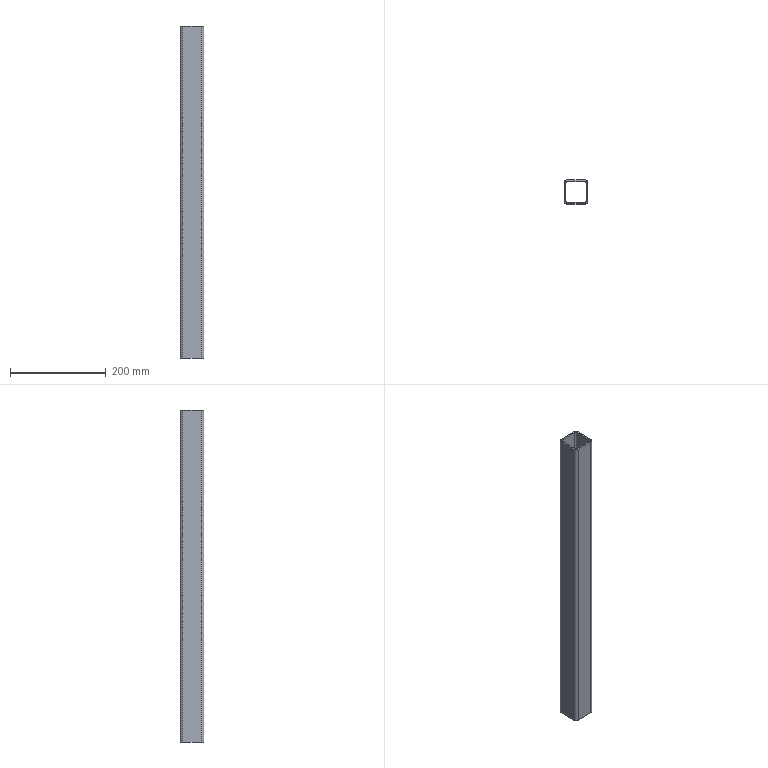Part | SolidWorks | 1 solid | 18 faces | box 50 x 50 x 695 mm | volume 375872 mm3 | plane 10 | cylinder 8 | commonest cylinder face diameters 6 x4 12 x4
STEP:
#1=CARTESIAN_POINT('',(19.,25.,347.5));
#2=VERTEX_POINT('',#1);
#3=CARTESIAN_POINT('',(25.,19.,347.5));
#4=VERTEX_POINT('',#3);
#5=CARTESIAN_POINT('',(19.,19.,347.5));
#6=DIRECTION('',(0.,0.,-1.));
#7=DIRECTION('',(-1.,0.,0.));
#8=AXIS2_PLACEMENT_3D('',#5,#6,#7);
#9=CIRCLE('',#8,6.);
#10=EDGE_CURVE('',#2,#4,#9,.T.);
#11=ORIENTED_EDGE('',*,*,#10,.T.);
#12=CARTESIAN_POINT('',(25.,19.,-347.5));
#13=VERTEX_POINT('',#12);
#14=CARTESIAN_POINT('',(25.,19.,-347.5));
#15=DIRECTION('',(0.,0.,1.));
#16=VECTOR('',#15,1000.);
#17=LINE('',#14,#16);
#18=EDGE_CURVE('',#13,#4,#17,.T.);
#19=ORIENTED_EDGE('',*,*,#18,.F.);
#20=CARTESIAN_POINT('',(19.,25.,-347.5));
#21=VERTEX_POINT('',#20);
#22=CARTESIAN_POINT('',(19.,19.,-347.5));
#23=DIRECTION('',(0.,0.,-1.));
#24=DIRECTION('',(-1.,0.,0.));
#25=AXIS2_PLACEMENT_3D('',#22,#23,#24);
#26=CIRCLE('',#25,6.);
#27=EDGE_CURVE('',#21,#13,#26,.T.);
#28=ORIENTED_EDGE('',*,*,#27,.F.);
#29=CARTESIAN_POINT('',(19.,25.,-347.5));
#30=DIRECTION('',(0.,0.,1.));
#31=VECTOR('',#30,1000.);
#32=LINE('',#29,#31);
#33=EDGE_CURVE('',#21,#2,#32,.T.);
#34=ORIENTED_EDGE('',*,*,#33,.T.);
#35=EDGE_LOOP('',(#11,#19,#28,#34));
#36=FACE_OUTER_BOUND('',#35,.T.);
#37=CARTESIAN_POINT('',(19.,19.,-347.5));
#38=DIRECTION('',(0.,0.,1.));
#39=DIRECTION('',(1.,0.,0.));
#40=AXIS2_PLACEMENT_3D('',#37,#38,#39);
#41=CYLINDRICAL_SURFACE('',#40,6.);
#42=ADVANCED_FACE('',(#36),#41,.T.);
#43=CARTESIAN_POINT('',(25.,-19.,347.5));
#44=VERTEX_POINT('',#43);
#45=CARTESIAN_POINT('',(25.,19.,347.5));
#46=DIRECTION('',(0.,-1.,0.));
#47=VECTOR('',#46,1000.);
#48=LINE('',#45,#47);
#49=EDGE_CURVE('',#4,#44,#48,.T.);
#50=ORIENTED_EDGE('',*,*,#49,.T.);
#51=CARTESIAN_POINT('',(25.,-19.,-347.5));
#52=VERTEX_POINT('',#51);
#53=CARTESIAN_POINT('',(25.,-19.,-347.5));
#54=DIRECTION('',(0.,0.,1.));
#55=VECTOR('',#54,1000.);
#56=LINE('',#53,#55);
#57=EDGE_CURVE('',#52,#44,#56,.T.);
#58=ORIENTED_EDGE('',*,*,#57,.F.);
#59=CARTESIAN_POINT('',(25.,19.,-347.5));
#60=DIRECTION('',(0.,-1.,0.));
#61=VECTOR('',#60,1000.);
#62=LINE('',#59,#61);
#63=EDGE_CURVE('',#13,#52,#62,.T.);
#64=ORIENTED_EDGE('',*,*,#63,.F.);
#65=ORIENTED_EDGE('',*,*,#18,.T.);
#66=EDGE_LOOP('',(#50,#58,#64,#65));
#67=FACE_OUTER_BOUND('',#66,.T.);
#68=CARTESIAN_POINT('',(25.,19.,-347.5));
#69=DIRECTION('',(-1.,0.,0.));
#70=DIRECTION('',(0.,0.,1.));
#71=AXIS2_PLACEMENT_3D('',#68,#69,#70);
#72=PLANE('',#71);
#73=ADVANCED_FACE('',(#67),#72,.F.);
#74=CARTESIAN_POINT('',(19.,-25.,347.5));
#75=VERTEX_POINT('',#74);
#76=CARTESIAN_POINT('',(19.,-19.,347.5));
#77=DIRECTION('',(0.,0.,-1.));
#78=DIRECTION('',(-1.,0.,0.));
#79=AXIS2_PLACEMENT_3D('',#76,#77,#78);
#80=CIRCLE('',#79,6.);
#81=EDGE_CURVE('',#44,#75,#80,.T.);
#82=ORIENTED_EDGE('',*,*,#81,.T.);
#83=CARTESIAN_POINT('',(19.,-25.,-347.5));
#84=VERTEX_POINT('',#83);
#85=CARTESIAN_POINT('',(19.,-25.,-347.5));
#86=DIRECTION('',(0.,0.,1.));
#87=VECTOR('',#86,1000.);
#88=LINE('',#85,#87);
#89=EDGE_CURVE('',#84,#75,#88,.T.);
#90=ORIENTED_EDGE('',*,*,#89,.F.);
#91=CARTESIAN_POINT('',(19.,-19.,-347.5));
#92=DIRECTION('',(0.,0.,-1.));
#93=DIRECTION('',(-1.,0.,0.));
#94=AXIS2_PLACEMENT_3D('',#91,#92,#93);
#95=CIRCLE('',#94,6.);
#96=EDGE_CURVE('',#52,#84,#95,.T.);
#97=ORIENTED_EDGE('',*,*,#96,.F.);
#98=ORIENTED_EDGE('',*,*,#57,.T.);
#99=EDGE_LOOP('',(#82,#90,#97,#98));
#100=FACE_OUTER_BOUND('',#99,.T.);
#101=CARTESIAN_POINT('',(19.,-19.,-347.5));
#102=DIRECTION('',(0.,0.,1.));
#103=DIRECTION('',(1.,0.,0.));
#104=AXIS2_PLACEMENT_3D('',#101,#102,#103);
#105=CYLINDRICAL_SURFACE('',#104,6.);
#106=ADVANCED_FACE('',(#100),#105,.T.);
#107=CARTESIAN_POINT('',(-19.,-25.,347.5));
#108=VERTEX_POINT('',#107);
#109=CARTESIAN_POINT('',(-19.,-25.,347.5));
#110=DIRECTION('',(-1.,0.,0.));
#111=VECTOR('',#110,1000.);
#112=LINE('',#109,#111);
#113=EDGE_CURVE('',#75,#108,#112,.T.);
#114=ORIENTED_EDGE('',*,*,#113,.T.);
#115=CARTESIAN_POINT('',(-19.,-25.,-347.5));
#116=VERTEX_POINT('',#115);
#117=CARTESIAN_POINT('',(-19.,-25.,-347.5));
#118=DIRECTION('',(0.,0.,1.));
#119=VECTOR('',#118,1000.);
#120=LINE('',#117,#119);
#121=EDGE_CURVE('',#116,#108,#120,.T.);
#122=ORIENTED_EDGE('',*,*,#121,.F.);
#123=CARTESIAN_POINT('',(-19.,-25.,-347.5));
#124=DIRECTION('',(-1.,0.,0.));
#125=VECTOR('',#124,1000.);
#126=LINE('',#123,#125);
#127=EDGE_CURVE('',#84,#116,#126,.T.);
#128=ORIENTED_EDGE('',*,*,#127,.F.);
#129=ORIENTED_EDGE('',*,*,#89,.T.);
#130=EDGE_LOOP('',(#114,#122,#128,#129));
#131=FACE_OUTER_BOUND('',#130,.T.);
#132=CARTESIAN_POINT('',(-19.,-25.,-347.5));
#133=DIRECTION('',(0.,1.,0.));
#134=DIRECTION('',(0.,0.,1.));
#135=AXIS2_PLACEMENT_3D('',#132,#133,#134);
#136=PLANE('',#135);
#137=ADVANCED_FACE('',(#131),#136,.F.);
#138=CARTESIAN_POINT('',(-25.,-19.,347.5));
#139=VERTEX_POINT('',#138);
#140=CARTESIAN_POINT('',(-19.,-19.,347.5));
#141=DIRECTION('',(0.,0.,-1.));
#142=DIRECTION('',(-1.,0.,0.));
#143=AXIS2_PLACEMENT_3D('',#140,#141,#142);
#144=CIRCLE('',#143,6.);
#145=EDGE_CURVE('',#108,#139,#144,.T.);
#146=ORIENTED_EDGE('',*,*,#145,.T.);
#147=CARTESIAN_POINT('',(-25.,-19.,-347.5));
#148=VERTEX_POINT('',#147);
#149=CARTESIAN_POINT('',(-25.,-19.,-347.5));
#150=DIRECTION('',(0.,0.,1.));
#151=VECTOR('',#150,1000.);
#152=LINE('',#149,#151);
#153=EDGE_CURVE('',#148,#139,#152,.T.);
#154=ORIENTED_EDGE('',*,*,#153,.F.);
#155=CARTESIAN_POINT('',(-19.,-19.,-347.5));
#156=DIRECTION('',(0.,0.,-1.));
#157=DIRECTION('',(-1.,0.,0.));
#158=AXIS2_PLACEMENT_3D('',#155,#156,#157);
#159=CIRCLE('',#158,6.);
#160=EDGE_CURVE('',#116,#148,#159,.T.);
#161=ORIENTED_EDGE('',*,*,#160,.F.);
#162=ORIENTED_EDGE('',*,*,#121,.T.);
#163=EDGE_LOOP('',(#146,#154,#161,#162));
#164=FACE_OUTER_BOUND('',#163,.T.);
#165=CARTESIAN_POINT('',(-19.,-19.,-347.5));
#166=DIRECTION('',(0.,0.,1.));
#167=DIRECTION('',(1.,0.,0.));
#168=AXIS2_PLACEMENT_3D('',#165,#166,#167);
#169=CYLINDRICAL_SURFACE('',#168,6.);
#170=ADVANCED_FACE('',(#164),#169,.T.);
#171=CARTESIAN_POINT('',(-25.,19.,347.5));
#172=VERTEX_POINT('',#171);
#173=CARTESIAN_POINT('',(-25.,-19.,347.5));
#174=DIRECTION('',(0.,1.,0.));
#175=VECTOR('',#174,1000.);
#176=LINE('',#173,#175);
#177=EDGE_CURVE('',#139,#172,#176,.T.);
#178=ORIENTED_EDGE('',*,*,#177,.T.);
#179=CARTESIAN_POINT('',(-25.,19.,-347.5));
#180=VERTEX_POINT('',#179);
#181=CARTESIAN_POINT('',(-25.,19.,-347.5));
#182=DIRECTION('',(0.,0.,1.));
#183=VECTOR('',#182,1000.);
#184=LINE('',#181,#183);
#185=EDGE_CURVE('',#180,#172,#184,.T.);
#186=ORIENTED_EDGE('',*,*,#185,.F.);
#187=CARTESIAN_POINT('',(-25.,-19.,-347.5));
#188=DIRECTION('',(0.,1.,0.));
#189=VECTOR('',#188,1000.);
#190=LINE('',#187,#189);
#191=EDGE_CURVE('',#148,#180,#190,.T.);
#192=ORIENTED_EDGE('',*,*,#191,.F.);
#193=ORIENTED_EDGE('',*,*,#153,.T.);
#194=EDGE_LOOP('',(#178,#186,#192,#193));
#195=FACE_OUTER_BOUND('',#194,.T.);
#196=CARTESIAN_POINT('',(-25.,-19.,-347.5));
#197=DIRECTION('',(1.,0.,0.));
#198=DIRECTION('',(0.,0.,-1.));
#199=AXIS2_PLACEMENT_3D('',#196,#197,#198);
#200=PLANE('',#199);
#201=ADVANCED_FACE('',(#195),#200,.F.);
#202=CARTESIAN_POINT('',(-19.,25.,347.5));
#203=VERTEX_POINT('',#202);
#204=CARTESIAN_POINT('',(-19.,19.,347.5));
#205=DIRECTION('',(0.,0.,-1.));
#206=DIRECTION('',(-1.,0.,0.));
#207=AXIS2_PLACEMENT_3D('',#204,#205,#206);
#208=CIRCLE('',#207,6.);
#209=EDGE_CURVE('',#172,#203,#208,.T.);
#210=ORIENTED_EDGE('',*,*,#209,.T.);
#211=CARTESIAN_POINT('',(-19.,25.,-347.5));
#212=VERTEX_POINT('',#211);
#213=CARTESIAN_POINT('',(-19.,25.,-347.5));
#214=DIRECTION('',(0.,0.,1.));
#215=VECTOR('',#214,1000.);
#216=LINE('',#213,#215);
#217=EDGE_CURVE('',#212,#203,#216,.T.);
#218=ORIENTED_EDGE('',*,*,#217,.F.);
#219=CARTESIAN_POINT('',(-19.,19.,-347.5));
#220=DIRECTION('',(0.,0.,-1.));
#221=DIRECTION('',(-1.,0.,0.));
#222=AXIS2_PLACEMENT_3D('',#219,#220,#221);
#223=CIRCLE('',#222,6.);
#224=EDGE_CURVE('',#180,#212,#223,.T.);
#225=ORIENTED_EDGE('',*,*,#224,.F.);
#226=ORIENTED_EDGE('',*,*,#185,.T.);
#227=EDGE_LOOP('',(#210,#218,#225,#226));
#228=FACE_OUTER_BOUND('',#227,.T.);
#229=CARTESIAN_POINT('',(-19.,19.,-347.5));
#230=DIRECTION('',(0.,0.,1.));
#231=DIRECTION('',(1.,0.,0.));
#232=AXIS2_PLACEMENT_3D('',#229,#230,#231);
#233=CYLINDRICAL_SURFACE('',#232,6.);
#234=ADVANCED_FACE('',(#228),#233,.T.);
#235=CARTESIAN_POINT('',(22.,-19.,347.5));
#236=VERTEX_POINT('',#235);
#237=CARTESIAN_POINT('',(19.,-22.,347.5));
#238=VERTEX_POINT('',#237);
#239=CARTESIAN_POINT('',(19.,-19.,347.5));
#240=DIRECTION('',(0.,0.,-1.));
#241=DIRECTION('',(-1.,0.,0.));
#242=AXIS2_PLACEMENT_3D('',#239,#240,#241);
#243=CIRCLE('',#242,3.);
#244=EDGE_CURVE('',#236,#238,#243,.T.);
#245=ORIENTED_EDGE('',*,*,#244,.F.);
#246=CARTESIAN_POINT('',(22.,-19.,-347.5));
#247=VERTEX_POINT('',#246);
#248=CARTESIAN_POINT('',(22.,-19.,-347.5));
#249=DIRECTION('',(0.,0.,1.));
#250=VECTOR('',#249,1000.);
#251=LINE('',#248,#250);
#252=EDGE_CURVE('',#247,#236,#251,.T.);
#253=ORIENTED_EDGE('',*,*,#252,.F.);
#254=CARTESIAN_POINT('',(19.,-22.,-347.5));
#255=VERTEX_POINT('',#254);
#256=CARTESIAN_POINT('',(19.,-19.,-347.5));
#257=DIRECTION('',(0.,0.,-1.));
#258=DIRECTION('',(-1.,0.,0.));
#259=AXIS2_PLACEMENT_3D('',#256,#257,#258);
#260=CIRCLE('',#259,3.);
#261=EDGE_CURVE('',#247,#255,#260,.T.);
#262=ORIENTED_EDGE('',*,*,#261,.T.);
#263=CARTESIAN_POINT('',(19.,-22.,-347.5));
#264=DIRECTION('',(0.,0.,1.));
#265=VECTOR('',#264,1000.);
#266=LINE('',#263,#265);
#267=EDGE_CURVE('',#255,#238,#266,.T.);
#268=ORIENTED_EDGE('',*,*,#267,.T.);
#269=EDGE_LOOP('',(#245,#253,#262,#268));
#270=FACE_OUTER_BOUND('',#269,.T.);
#271=CARTESIAN_POINT('',(19.,-19.,-347.5));
#272=DIRECTION('',(0.,0.,1.));
#273=DIRECTION('',(1.,0.,0.));
#274=AXIS2_PLACEMENT_3D('',#271,#272,#273);
#275=CYLINDRICAL_SURFACE('',#274,3.);
#276=ADVANCED_FACE('',(#270),#275,.F.);
#277=CARTESIAN_POINT('',(22.,19.,347.5));
#278=VERTEX_POINT('',#277);
#279=CARTESIAN_POINT('',(22.,19.,347.5));
#280=DIRECTION('',(0.,-1.,0.));
#281=VECTOR('',#280,1000.);
#282=LINE('',#279,#281);
#283=EDGE_CURVE('',#278,#236,#282,.T.);
#284=ORIENTED_EDGE('',*,*,#283,.F.);
#285=CARTESIAN_POINT('',(22.,19.,-347.5));
#286=VERTEX_POINT('',#285);
#287=CARTESIAN_POINT('',(22.,19.,-347.5));
#288=DIRECTION('',(0.,0.,1.));
#289=VECTOR('',#288,1000.);
#290=LINE('',#287,#289);
#291=EDGE_CURVE('',#286,#278,#290,.T.);
#292=ORIENTED_EDGE('',*,*,#291,.F.);
#293=CARTESIAN_POINT('',(22.,19.,-347.5));
#294=DIRECTION('',(0.,-1.,0.));
#295=VECTOR('',#294,1000.);
#296=LINE('',#293,#295);
#297=EDGE_CURVE('',#286,#247,#296,.T.);
#298=ORIENTED_EDGE('',*,*,#297,.T.);
#299=ORIENTED_EDGE('',*,*,#252,.T.);
#300=EDGE_LOOP('',(#284,#292,#298,#299));
#301=FACE_OUTER_BOUND('',#300,.T.);
#302=CARTESIAN_POINT('',(22.,19.,-347.5));
#303=DIRECTION('',(-1.,0.,0.));
#304=DIRECTION('',(0.,0.,1.));
#305=AXIS2_PLACEMENT_3D('',#302,#303,#304);
#306=PLANE('',#305);
#307=ADVANCED_FACE('',(#301),#306,.T.);
#308=CARTESIAN_POINT('',(19.,22.,347.5));
#309=VERTEX_POINT('',#308);
#310=CARTESIAN_POINT('',(19.,19.,347.5));
#311=DIRECTION('',(0.,0.,-1.));
#312=DIRECTION('',(-1.,0.,0.));
#313=AXIS2_PLACEMENT_3D('',#310,#311,#312);
#314=CIRCLE('',#313,3.);
#315=EDGE_CURVE('',#309,#278,#314,.T.);
#316=ORIENTED_EDGE('',*,*,#315,.F.);
#317=CARTESIAN_POINT('',(19.,22.,-347.5));
#318=VERTEX_POINT('',#317);
#319=CARTESIAN_POINT('',(19.,22.,-347.5));
#320=DIRECTION('',(0.,0.,1.));
#321=VECTOR('',#320,1000.);
#322=LINE('',#319,#321);
#323=EDGE_CURVE('',#318,#309,#322,.T.);
#324=ORIENTED_EDGE('',*,*,#323,.F.);
#325=CARTESIAN_POINT('',(19.,19.,-347.5));
#326=DIRECTION('',(0.,0.,-1.));
#327=DIRECTION('',(-1.,0.,0.));
#328=AXIS2_PLACEMENT_3D('',#325,#326,#327);
#329=CIRCLE('',#328,3.);
#330=EDGE_CURVE('',#318,#286,#329,.T.);
#331=ORIENTED_EDGE('',*,*,#330,.T.);
#332=ORIENTED_EDGE('',*,*,#291,.T.);
#333=EDGE_LOOP('',(#316,#324,#331,#332));
#334=FACE_OUTER_BOUND('',#333,.T.);
#335=CARTESIAN_POINT('',(19.,19.,-347.5));
#336=DIRECTION('',(0.,0.,1.));
#337=DIRECTION('',(1.,0.,0.));
#338=AXIS2_PLACEMENT_3D('',#335,#336,#337);
#339=CYLINDRICAL_SURFACE('',#338,3.);
#340=ADVANCED_FACE('',(#334),#339,.F.);
#341=CARTESIAN_POINT('',(-19.,22.,347.5));
#342=VERTEX_POINT('',#341);
#343=CARTESIAN_POINT('',(19.,22.,347.5));
#344=DIRECTION('',(1.,0.,0.));
#345=VECTOR('',#344,1000.);
#346=LINE('',#343,#345);
#347=EDGE_CURVE('',#342,#309,#346,.T.);
#348=ORIENTED_EDGE('',*,*,#347,.F.);
#349=CARTESIAN_POINT('',(-19.,22.,-347.5));
#350=VERTEX_POINT('',#349);
#351=CARTESIAN_POINT('',(-19.,22.,-347.5));
#352=DIRECTION('',(0.,0.,1.));
#353=VECTOR('',#352,1000.);
#354=LINE('',#351,#353);
#355=EDGE_CURVE('',#350,#342,#354,.T.);
#356=ORIENTED_EDGE('',*,*,#355,.F.);
#357=CARTESIAN_POINT('',(19.,22.,-347.5));
#358=DIRECTION('',(1.,0.,0.));
#359=VECTOR('',#358,1000.);
#360=LINE('',#357,#359);
#361=EDGE_CURVE('',#350,#318,#360,.T.);
#362=ORIENTED_EDGE('',*,*,#361,.T.);
#363=ORIENTED_EDGE('',*,*,#323,.T.);
#364=EDGE_LOOP('',(#348,#356,#362,#363));
#365=FACE_OUTER_BOUND('',#364,.T.);
#366=CARTESIAN_POINT('',(19.,22.,-347.5));
#367=DIRECTION('',(0.,-1.,0.));
#368=DIRECTION('',(0.,0.,-1.));
#369=AXIS2_PLACEMENT_3D('',#366,#367,#368);
#370=PLANE('',#369);
#371=ADVANCED_FACE('',(#365),#370,.T.);
#372=CARTESIAN_POINT('',(-22.,19.,347.5));
#373=VERTEX_POINT('',#372);
#374=CARTESIAN_POINT('',(-19.,19.,347.5));
#375=DIRECTION('',(0.,0.,-1.));
#376=DIRECTION('',(-1.,0.,0.));
#377=AXIS2_PLACEMENT_3D('',#374,#375,#376);
#378=CIRCLE('',#377,3.);
#379=EDGE_CURVE('',#373,#342,#378,.T.);
#380=ORIENTED_EDGE('',*,*,#379,.F.);
#381=CARTESIAN_POINT('',(-22.,19.,-347.5));
#382=VERTEX_POINT('',#381);
#383=CARTESIAN_POINT('',(-22.,19.,-347.5));
#384=DIRECTION('',(0.,0.,1.));
#385=VECTOR('',#384,1000.);
#386=LINE('',#383,#385);
#387=EDGE_CURVE('',#382,#373,#386,.T.);
#388=ORIENTED_EDGE('',*,*,#387,.F.);
#389=CARTESIAN_POINT('',(-19.,19.,-347.5));
#390=DIRECTION('',(0.,0.,-1.));
#391=DIRECTION('',(-1.,0.,0.));
#392=AXIS2_PLACEMENT_3D('',#389,#390,#391);
#393=CIRCLE('',#392,3.);
#394=EDGE_CURVE('',#382,#350,#393,.T.);
#395=ORIENTED_EDGE('',*,*,#394,.T.);
#396=ORIENTED_EDGE('',*,*,#355,.T.);
#397=EDGE_LOOP('',(#380,#388,#395,#396));
#398=FACE_OUTER_BOUND('',#397,.T.);
#399=CARTESIAN_POINT('',(-19.,19.,-347.5));
#400=DIRECTION('',(0.,0.,1.));
#401=DIRECTION('',(1.,0.,0.));
#402=AXIS2_PLACEMENT_3D('',#399,#400,#401);
#403=CYLINDRICAL_SURFACE('',#402,3.);
#404=ADVANCED_FACE('',(#398),#403,.F.);
#405=CARTESIAN_POINT('',(-22.,-19.,347.5));
#406=VERTEX_POINT('',#405);
#407=CARTESIAN_POINT('',(-22.,-19.,347.5));
#408=DIRECTION('',(0.,1.,0.));
#409=VECTOR('',#408,1000.);
#410=LINE('',#407,#409);
#411=EDGE_CURVE('',#406,#373,#410,.T.);
#412=ORIENTED_EDGE('',*,*,#411,.F.);
#413=CARTESIAN_POINT('',(-22.,-19.,-347.5));
#414=VERTEX_POINT('',#413);
#415=CARTESIAN_POINT('',(-22.,-19.,-347.5));
#416=DIRECTION('',(0.,0.,1.));
#417=VECTOR('',#416,1000.);
#418=LINE('',#415,#417);
#419=EDGE_CURVE('',#414,#406,#418,.T.);
#420=ORIENTED_EDGE('',*,*,#419,.F.);
#421=CARTESIAN_POINT('',(-22.,-19.,-347.5));
#422=DIRECTION('',(0.,1.,0.));
#423=VECTOR('',#422,1000.);
#424=LINE('',#421,#423);
#425=EDGE_CURVE('',#414,#382,#424,.T.);
#426=ORIENTED_EDGE('',*,*,#425,.T.);
#427=ORIENTED_EDGE('',*,*,#387,.T.);
#428=EDGE_LOOP('',(#412,#420,#426,#427));
#429=FACE_OUTER_BOUND('',#428,.T.);
#430=CARTESIAN_POINT('',(-22.,-19.,-347.5));
#431=DIRECTION('',(1.,0.,0.));
#432=DIRECTION('',(0.,0.,-1.));
#433=AXIS2_PLACEMENT_3D('',#430,#431,#432);
#434=PLANE('',#433);
#435=ADVANCED_FACE('',(#429),#434,.T.);
#436=CARTESIAN_POINT('',(-19.,-22.,347.5));
#437=VERTEX_POINT('',#436);
#438=CARTESIAN_POINT('',(-19.,-19.,347.5));
#439=DIRECTION('',(0.,0.,-1.));
#440=DIRECTION('',(-1.,0.,0.));
#441=AXIS2_PLACEMENT_3D('',#438,#439,#440);
#442=CIRCLE('',#441,3.);
#443=EDGE_CURVE('',#437,#406,#442,.T.);
#444=ORIENTED_EDGE('',*,*,#443,.F.);
#445=CARTESIAN_POINT('',(-19.,-22.,-347.5));
#446=VERTEX_POINT('',#445);
#447=CARTESIAN_POINT('',(-19.,-22.,-347.5));
#448=DIRECTION('',(0.,0.,1.));
#449=VECTOR('',#448,1000.);
#450=LINE('',#447,#449);
#451=EDGE_CURVE('',#446,#437,#450,.T.);
#452=ORIENTED_EDGE('',*,*,#451,.F.);
#453=CARTESIAN_POINT('',(-19.,-19.,-347.5));
#454=DIRECTION('',(0.,0.,-1.));
#455=DIRECTION('',(-1.,0.,0.));
#456=AXIS2_PLACEMENT_3D('',#453,#454,#455);
#457=CIRCLE('',#456,3.);
#458=EDGE_CURVE('',#446,#414,#457,.T.);
#459=ORIENTED_EDGE('',*,*,#458,.T.);
#460=ORIENTED_EDGE('',*,*,#419,.T.);
#461=EDGE_LOOP('',(#444,#452,#459,#460));
#462=FACE_OUTER_BOUND('',#461,.T.);
#463=CARTESIAN_POINT('',(-19.,-19.,-347.5));
#464=DIRECTION('',(0.,0.,1.));
#465=DIRECTION('',(1.,0.,0.));
#466=AXIS2_PLACEMENT_3D('',#463,#464,#465);
#467=CYLINDRICAL_SURFACE('',#466,3.);
#468=ADVANCED_FACE('',(#462),#467,.F.);
#469=CARTESIAN_POINT('',(-19.,-22.,347.5));
#470=DIRECTION('',(-1.,0.,0.));
#471=VECTOR('',#470,1000.);
#472=LINE('',#469,#471);
#473=EDGE_CURVE('',#238,#437,#472,.T.);
#474=ORIENTED_EDGE('',*,*,#473,.F.);
#475=ORIENTED_EDGE('',*,*,#267,.F.);
#476=CARTESIAN_POINT('',(-19.,-22.,-347.5));
#477=DIRECTION('',(-1.,0.,0.));
#478=VECTOR('',#477,1000.);
#479=LINE('',#476,#478);
#480=EDGE_CURVE('',#255,#446,#479,.T.);
#481=ORIENTED_EDGE('',*,*,#480,.T.);
#482=ORIENTED_EDGE('',*,*,#451,.T.);
#483=EDGE_LOOP('',(#474,#475,#481,#482));
#484=FACE_OUTER_BOUND('',#483,.T.);
#485=CARTESIAN_POINT('',(-19.,-22.,-347.5));
#486=DIRECTION('',(0.,1.,0.));
#487=DIRECTION('',(0.,0.,1.));
#488=AXIS2_PLACEMENT_3D('',#485,#486,#487);
#489=PLANE('',#488);
#490=ADVANCED_FACE('',(#484),#489,.T.);
#491=CARTESIAN_POINT('',(19.,25.,347.5));
#492=DIRECTION('',(1.,0.,0.));
#493=VECTOR('',#492,1000.);
#494=LINE('',#491,#493);
#495=EDGE_CURVE('',#203,#2,#494,.T.);
#496=ORIENTED_EDGE('',*,*,#495,.T.);
#497=ORIENTED_EDGE('',*,*,#33,.F.);
#498=CARTESIAN_POINT('',(19.,25.,-347.5));
#499=DIRECTION('',(1.,0.,0.));
#500=VECTOR('',#499,1000.);
#501=LINE('',#498,#500);
#502=EDGE_CURVE('',#212,#21,#501,.T.);
#503=ORIENTED_EDGE('',*,*,#502,.F.);
#504=ORIENTED_EDGE('',*,*,#217,.T.);
#505=EDGE_LOOP('',(#496,#497,#503,#504));
#506=FACE_OUTER_BOUND('',#505,.T.);
#507=CARTESIAN_POINT('',(19.,25.,-347.5));
#508=DIRECTION('',(0.,-1.,0.));
#509=DIRECTION('',(0.,0.,-1.));
#510=AXIS2_PLACEMENT_3D('',#507,#508,#509);
#511=PLANE('',#510);
#512=ADVANCED_FACE('',(#506),#511,.F.);
#513=ORIENTED_EDGE('',*,*,#261,.F.);
#514=ORIENTED_EDGE('',*,*,#297,.F.);
#515=ORIENTED_EDGE('',*,*,#330,.F.);
#516=ORIENTED_EDGE('',*,*,#361,.F.);
#517=ORIENTED_EDGE('',*,*,#394,.F.);
#518=ORIENTED_EDGE('',*,*,#425,.F.);
#519=ORIENTED_EDGE('',*,*,#458,.F.);
#520=ORIENTED_EDGE('',*,*,#480,.F.);
#521=EDGE_LOOP('',(#513,#514,#515,#516,#517,#518,#519,#520));
#522=FACE_BOUND('',#521,.T.);
#523=ORIENTED_EDGE('',*,*,#27,.T.);
#524=ORIENTED_EDGE('',*,*,#63,.T.);
#525=ORIENTED_EDGE('',*,*,#96,.T.);
#526=ORIENTED_EDGE('',*,*,#127,.T.);
#527=ORIENTED_EDGE('',*,*,#160,.T.);
#528=ORIENTED_EDGE('',*,*,#191,.T.);
#529=ORIENTED_EDGE('',*,*,#224,.T.);
#530=ORIENTED_EDGE('',*,*,#502,.T.);
#531=EDGE_LOOP('',(#523,#524,#525,#526,#527,#528,#529,#530));
#532=FACE_OUTER_BOUND('',#531,.T.);
#533=CARTESIAN_POINT('',(19.,19.,-347.5));
#534=DIRECTION('',(0.,0.,-1.));
#535=DIRECTION('',(-1.,0.,0.));
#536=AXIS2_PLACEMENT_3D('',#533,#534,#535);
#537=PLANE('',#536);
#538=ADVANCED_FACE('',(#522,#532),#537,.T.);
#539=ORIENTED_EDGE('',*,*,#244,.T.);
#540=ORIENTED_EDGE('',*,*,#473,.T.);
#541=ORIENTED_EDGE('',*,*,#443,.T.);
#542=ORIENTED_EDGE('',*,*,#411,.T.);
#543=ORIENTED_EDGE('',*,*,#379,.T.);
#544=ORIENTED_EDGE('',*,*,#347,.T.);
#545=ORIENTED_EDGE('',*,*,#315,.T.);
#546=ORIENTED_EDGE('',*,*,#283,.T.);
#547=EDGE_LOOP('',(#539,#540,#541,#542,#543,#544,#545,#546));
#548=FACE_BOUND('',#547,.T.);
#549=ORIENTED_EDGE('',*,*,#10,.F.);
#550=ORIENTED_EDGE('',*,*,#495,.F.);
#551=ORIENTED_EDGE('',*,*,#209,.F.);
#552=ORIENTED_EDGE('',*,*,#177,.F.);
#553=ORIENTED_EDGE('',*,*,#145,.F.);
#554=ORIENTED_EDGE('',*,*,#113,.F.);
#555=ORIENTED_EDGE('',*,*,#81,.F.);
#556=ORIENTED_EDGE('',*,*,#49,.F.);
#557=EDGE_LOOP('',(#549,#550,#551,#552,#553,#554,#555,#556));
#558=FACE_OUTER_BOUND('',#557,.T.);
#559=CARTESIAN_POINT('',(19.,19.,347.5));
#560=DIRECTION('',(0.,0.,-1.));
#561=DIRECTION('',(-1.,0.,0.));
#562=AXIS2_PLACEMENT_3D('',#559,#560,#561);
#563=PLANE('',#562);
#564=ADVANCED_FACE('',(#548,#558),#563,.F.);
#565=CLOSED_SHELL('',(#42,#73,#106,#137,#170,#201,#234,#276,#307,#340,#371,#404,#435,#468,#490,#512,#538,#564));
#566=MANIFOLD_SOLID_BREP('',#565);
#567=CARTESIAN_POINT('',(0.,0.,0.));
#568=DIRECTION('',(0.,0.,1.));
#569=DIRECTION('',(1.,0.,0.));
#570=AXIS2_PLACEMENT_3D('',#567,#568,#569);
#571=(LENGTH_UNIT()NAMED_UNIT(*)SI_UNIT(.MILLI.,.METRE.));
#572=UNCERTAINTY_MEASURE_WITH_UNIT(LENGTH_MEASURE(0.00001),#571,'','');
#573=(NAMED_UNIT(*)PLANE_ANGLE_UNIT()SI_UNIT($,.RADIAN.));
#574=(NAMED_UNIT(*)SI_UNIT($,.STERADIAN.)SOLID_ANGLE_UNIT());
#575=(GEOMETRIC_REPRESENTATION_CONTEXT(3)GLOBAL_UNCERTAINTY_ASSIGNED_CONTEXT((#572))GLOBAL_UNIT_ASSIGNED_CONTEXT((#571,#573,#574))REPRESENTATION_CONTEXT('',''));
#576=ADVANCED_BREP_SHAPE_REPRESENTATION('',(#566,#570),#575);